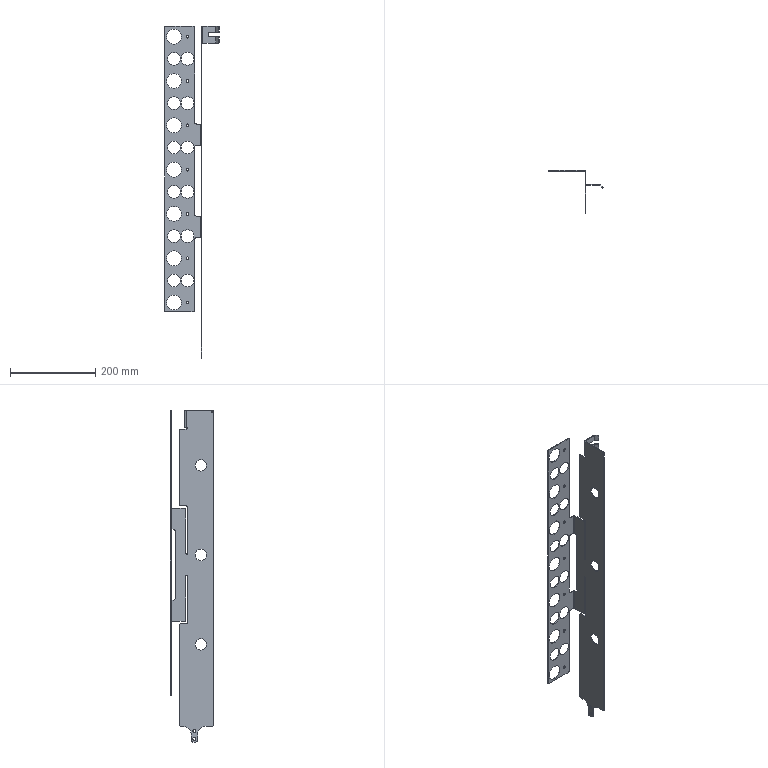Part | STEP file | 64524275 | 1 solid | 170 faces | box 128.478 x 101 x 779 mm | volume 142481 mm3 | cylinder 101 | plane 69 | commonest cylinder face diameters 30 x24 8 x23 35 x16 6.5 x14 27 x6 3 x5